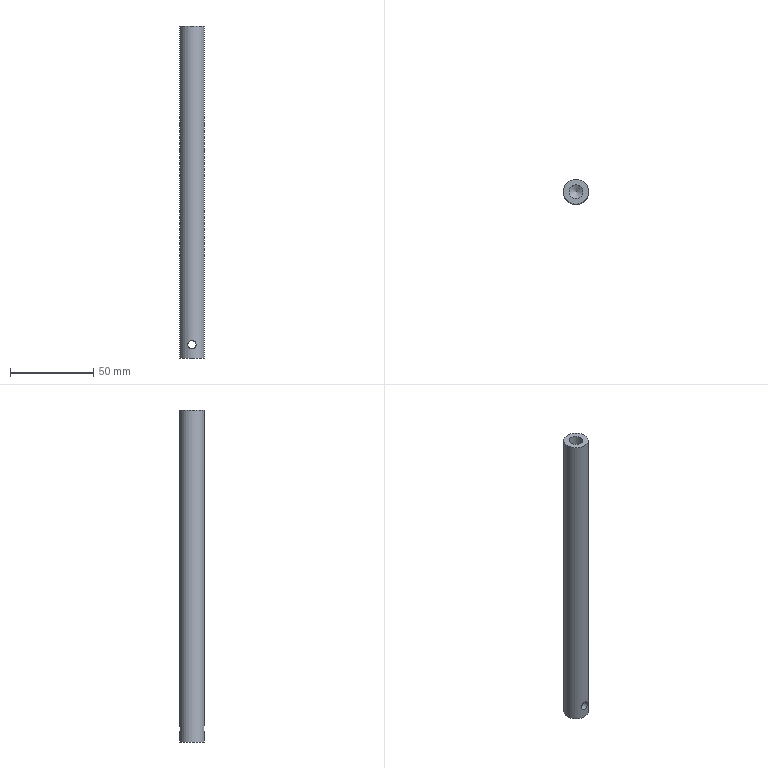Part | STEP file | axe for guide1-02 | 1 solid | 6 faces | box 15 x 15 x 200 mm | volume 33907 mm3 | spline 3 | plane 2 | cylinder 1 | commonest cylinder face diameters 15 x1
STEP:
#1=CARTESIAN_POINT('',(0.,0.,0.));
#2=DIRECTION('',(0.,0.,1.));
#3=DIRECTION('',(1.,0.,0.));
#4=AXIS2_PLACEMENT_3D('',#1,#2,#3);
#5=CARTESIAN_POINT('',(0.,7.5,10.5));
#6=VERTEX_POINT('',#5);
#7=CARTESIAN_POINT('',(0.,7.5,5.5));
#8=VERTEX_POINT('',#7);
#9=CARTESIAN_POINT('',(0.,7.5,10.5));
#10=CARTESIAN_POINT('',(-0.3165,7.5,10.5));
#11=CARTESIAN_POINT('',(-0.6524,7.478,10.436));
#12=CARTESIAN_POINT('',(-1.268,7.399,10.18));
#13=CARTESIAN_POINT('',(-1.547,7.342,9.988));
#14=CARTESIAN_POINT('',(-1.988,7.235,9.547));
#15=CARTESIAN_POINT('',(-2.18,7.177,9.268));
#16=CARTESIAN_POINT('',(-2.436,7.095,8.653));
#17=CARTESIAN_POINT('',(-2.5,7.071,8.317));
#18=CARTESIAN_POINT('',(-2.5,7.071,8.));
#19=CARTESIAN_POINT('',(-2.5,7.071,7.683));
#20=CARTESIAN_POINT('',(-2.436,7.095,7.347));
#21=CARTESIAN_POINT('',(-2.18,7.177,6.732));
#22=CARTESIAN_POINT('',(-1.988,7.235,6.453));
#23=CARTESIAN_POINT('',(-1.547,7.342,6.012));
#24=CARTESIAN_POINT('',(-1.268,7.399,5.82));
#25=CARTESIAN_POINT('',(-0.6524,7.478,5.564));
#26=CARTESIAN_POINT('',(-0.3165,7.5,5.5));
#27=CARTESIAN_POINT('',(0.,7.5,5.5));
#28=B_SPLINE_CURVE_WITH_KNOTS('',3,(#9,#10,#11,#12,#13,#14,#15,#16,#17,#18,#19,#20,#21,#22,#23,#24,#25,#26,#27),.UNSPECIFIED.,.F.,.F.,(4,2,2,2,3,2,2,2,4),(1.14,1.234,1.329,1.424,1.519,1.614,1.709,1.804,1.899),.UNSPECIFIED.);
#29=CARTESIAN_POINT('',(2.5,7.502,8.));
#30=CARTESIAN_POINT('',(2.5,7.502,5.5));
#31=CARTESIAN_POINT('',(0.,7.502,5.5));
#32=CARTESIAN_POINT('',(-2.5,7.502,5.5));
#33=CARTESIAN_POINT('',(-2.5,7.502,8.));
#34=CARTESIAN_POINT('',(-2.5,7.502,10.5));
#35=CARTESIAN_POINT('',(0.,7.502,10.5));
#36=CARTESIAN_POINT('',(2.5,7.502,10.5));
#37=CARTESIAN_POINT('',(2.5,7.502,8.));
#38=CARTESIAN_POINT('',(2.5,-7.502,8.));
#39=CARTESIAN_POINT('',(2.5,-7.502,5.5));
#40=CARTESIAN_POINT('',(0.,-7.502,5.5));
#41=CARTESIAN_POINT('',(-2.5,-7.502,5.5));
#42=CARTESIAN_POINT('',(-2.5,-7.502,8.));
#43=CARTESIAN_POINT('',(-2.5,-7.502,10.5));
#44=CARTESIAN_POINT('',(0.,-7.502,10.5));
#45=CARTESIAN_POINT('',(2.5,-7.502,10.5));
#46=CARTESIAN_POINT('',(2.5,-7.502,8.));
#47=(BOUNDED_SURFACE()B_SPLINE_SURFACE(1,2,((#29,#30,#31,#32,#33,#34,#35,#36,#37),(#38,#39,#40,#41,#42,#43,#44,#45,#46)),.UNSPECIFIED.,.F.,.T.,.F.)B_SPLINE_SURFACE_WITH_KNOTS((2,2),(1,2,2,2,2,2,1),(-80.449,-74.448),(-3.927,0.,3.927,7.854,11.781,15.708,19.635),.UNSPECIFIED.)GEOMETRIC_REPRESENTATION_ITEM()RATIONAL_B_SPLINE_SURFACE(((1.,0.7071,1.,0.7071,1.,0.7071,1.,0.7071,1.),(1.,0.7071,1.,0.7071,1.,0.7071,1.,0.7071,1.)))REPRESENTATION_ITEM('')SURFACE());
#48=CARTESIAN_POINT('',(-80.449,11.781));
#49=CARTESIAN_POINT('',(-80.449,11.717));
#50=CARTESIAN_POINT('',(-80.448,11.59));
#51=CARTESIAN_POINT('',(-80.446,11.4));
#52=CARTESIAN_POINT('',(-80.441,11.213));
#53=CARTESIAN_POINT('',(-80.436,11.028));
#54=CARTESIAN_POINT('',(-80.428,10.846));
#55=CARTESIAN_POINT('',(-80.42,10.667));
#56=CARTESIAN_POINT('',(-80.41,10.491));
#57=CARTESIAN_POINT('',(-80.399,10.317));
#58=CARTESIAN_POINT('',(-80.388,10.147));
#59=CARTESIAN_POINT('',(-80.376,9.98));
#60=CARTESIAN_POINT('',(-80.364,9.817));
#61=CARTESIAN_POINT('',(-80.352,9.655));
#62=CARTESIAN_POINT('',(-80.341,9.487));
#63=CARTESIAN_POINT('',(-80.329,9.317));
#64=CARTESIAN_POINT('',(-80.318,9.144));
#65=CARTESIAN_POINT('',(-80.308,8.968));
#66=CARTESIAN_POINT('',(-80.299,8.789));
#67=CARTESIAN_POINT('',(-80.291,8.607));
#68=CARTESIAN_POINT('',(-80.285,8.422));
#69=CARTESIAN_POINT('',(-80.281,8.235));
#70=CARTESIAN_POINT('',(-80.278,8.045));
#71=CARTESIAN_POINT('',(-80.277,7.854));
#72=CARTESIAN_POINT('',(-80.278,7.663));
#73=CARTESIAN_POINT('',(-80.281,7.473));
#74=CARTESIAN_POINT('',(-80.285,7.286));
#75=CARTESIAN_POINT('',(-80.291,7.101));
#76=CARTESIAN_POINT('',(-80.299,6.919));
#77=CARTESIAN_POINT('',(-80.308,6.74));
#78=CARTESIAN_POINT('',(-80.318,6.564));
#79=CARTESIAN_POINT('',(-80.329,6.391));
#80=CARTESIAN_POINT('',(-80.341,6.221));
#81=CARTESIAN_POINT('',(-80.352,6.053));
#82=CARTESIAN_POINT('',(-80.364,5.891));
#83=CARTESIAN_POINT('',(-80.376,5.728));
#84=CARTESIAN_POINT('',(-80.388,5.561));
#85=CARTESIAN_POINT('',(-80.399,5.391));
#86=CARTESIAN_POINT('',(-80.41,5.217));
#87=CARTESIAN_POINT('',(-80.42,5.041));
#88=CARTESIAN_POINT('',(-80.428,4.862));
#89=CARTESIAN_POINT('',(-80.436,4.68));
#90=CARTESIAN_POINT('',(-80.441,4.495));
#91=CARTESIAN_POINT('',(-80.446,4.308));
#92=CARTESIAN_POINT('',(-80.448,4.118));
#93=CARTESIAN_POINT('',(-80.449,3.991));
#94=CARTESIAN_POINT('',(-80.449,3.927));
#95=B_SPLINE_CURVE_WITH_KNOTS('',3,(#48,#49,#50,#51,#52,#53,#54,#55,#56,#57,#58,#59,#60,#61,#62,#63,#64,#65,#66,#67,#68,#69,#70,#71,#72,#73,#74,#75,#76,#77,#78,#79,#80,#81,#82,#83,#84,#85,#86,#87,#88,#89,#90,#91,#92,#93,#94),.UNSPECIFIED.,.F.,.F.,(4,1,1,1,1,1,1,1,1,1,1,1,1,1,1,1,1,1,1,1,1,1,1,1,1,1,1,1,1,1,1,1,1,1,1,1,1,1,1,1,1,1,1,1,4),(1.14,1.157,1.174,1.191,1.209,1.226,1.243,1.26,1.278,1.295,1.312,1.329,1.347,1.364,1.381,1.399,1.416,1.433,1.45,1.468,1.485,1.502,1.519,1.537,1.554,1.571,1.588,1.606,1.623,1.64,1.658,1.675,1.692,1.709,1.727,1.744,1.761,1.778,1.796,1.813,1.83,1.847,1.865,1.882,1.899),.QUASI_UNIFORM_KNOTS.);
#96=(GEOMETRIC_REPRESENTATION_CONTEXT(2)PARAMETRIC_REPRESENTATION_CONTEXT()REPRESENTATION_CONTEXT('',''));
#97=DEFINITIONAL_REPRESENTATION('',(#95),#96);
#98=PCURVE('',#47,#97);
#99=CARTESIAN_POINT('',(0.,0.,0.));
#100=DIRECTION('',(0.,0.,1.));
#101=DIRECTION('',(-1.,0.,0.));
#102=AXIS2_PLACEMENT_3D('',#99,#100,#101);
#103=CYLINDRICAL_SURFACE('',#102,7.5);
#104=CARTESIAN_POINT('',(4.712,10.5));
#105=CARTESIAN_POINT('',(4.72,10.5));
#106=CARTESIAN_POINT('',(4.736,10.496));
#107=CARTESIAN_POINT('',(4.759,10.477));
#108=CARTESIAN_POINT('',(4.783,10.445));
#109=CARTESIAN_POINT('',(4.806,10.401));
#110=CARTESIAN_POINT('',(4.83,10.344));
#111=CARTESIAN_POINT('',(4.852,10.274));
#112=CARTESIAN_POINT('',(4.874,10.192));
#113=CARTESIAN_POINT('',(4.895,10.099));
#114=CARTESIAN_POINT('',(4.915,9.997));
#115=CARTESIAN_POINT('',(4.933,9.886));
#116=CARTESIAN_POINT('',(4.951,9.769));
#117=CARTESIAN_POINT('',(4.967,9.643));
#118=CARTESIAN_POINT('',(4.982,9.506));
#119=CARTESIAN_POINT('',(4.996,9.36));
#120=CARTESIAN_POINT('',(5.009,9.206));
#121=CARTESIAN_POINT('',(5.02,9.044));
#122=CARTESIAN_POINT('',(5.03,8.876));
#123=CARTESIAN_POINT('',(5.038,8.703));
#124=CARTESIAN_POINT('',(5.044,8.528));
#125=CARTESIAN_POINT('',(5.049,8.351));
#126=CARTESIAN_POINT('',(5.052,8.174));
#127=CARTESIAN_POINT('',(5.053,8.));
#128=CARTESIAN_POINT('',(5.052,7.826));
#129=CARTESIAN_POINT('',(5.049,7.649));
#130=CARTESIAN_POINT('',(5.044,7.472));
#131=CARTESIAN_POINT('',(5.038,7.297));
#132=CARTESIAN_POINT('',(5.03,7.124));
#133=CARTESIAN_POINT('',(5.02,6.956));
#134=CARTESIAN_POINT('',(5.009,6.794));
#135=CARTESIAN_POINT('',(4.996,6.64));
#136=CARTESIAN_POINT('',(4.982,6.494));
#137=CARTESIAN_POINT('',(4.967,6.357));
#138=CARTESIAN_POINT('',(4.951,6.231));
#139=CARTESIAN_POINT('',(4.933,6.114));
#140=CARTESIAN_POINT('',(4.915,6.003));
#141=CARTESIAN_POINT('',(4.895,5.901));
#142=CARTESIAN_POINT('',(4.874,5.808));
#143=CARTESIAN_POINT('',(4.852,5.726));
#144=CARTESIAN_POINT('',(4.83,5.656));
#145=CARTESIAN_POINT('',(4.806,5.599));
#146=CARTESIAN_POINT('',(4.783,5.555));
#147=CARTESIAN_POINT('',(4.759,5.523));
#148=CARTESIAN_POINT('',(4.736,5.504));
#149=CARTESIAN_POINT('',(4.72,5.5));
#150=CARTESIAN_POINT('',(4.712,5.5));
#151=B_SPLINE_CURVE_WITH_KNOTS('',3,(#104,#105,#106,#107,#108,#109,#110,#111,#112,#113,#114,#115,#116,#117,#118,#119,#120,#121,#122,#123,#124,#125,#126,#127,#128,#129,#130,#131,#132,#133,#134,#135,#136,#137,#138,#139,#140,#141,#142,#143,#144,#145,#146,#147,#148,#149,#150),.UNSPECIFIED.,.F.,.F.,(4,1,1,1,1,1,1,1,1,1,1,1,1,1,1,1,1,1,1,1,1,1,1,1,1,1,1,1,1,1,1,1,1,1,1,1,1,1,1,1,1,1,1,1,4),(1.14,1.157,1.174,1.191,1.209,1.226,1.243,1.26,1.278,1.295,1.312,1.329,1.347,1.364,1.381,1.399,1.416,1.433,1.45,1.468,1.485,1.502,1.519,1.537,1.554,1.571,1.588,1.606,1.623,1.64,1.658,1.675,1.692,1.709,1.727,1.744,1.761,1.778,1.796,1.813,1.83,1.847,1.865,1.882,1.899),.QUASI_UNIFORM_KNOTS.);
#152=(GEOMETRIC_REPRESENTATION_CONTEXT(2)PARAMETRIC_REPRESENTATION_CONTEXT()REPRESENTATION_CONTEXT('',''));
#153=DEFINITIONAL_REPRESENTATION('',(#151),#152);
#154=PCURVE('',#103,#153);
#155=SURFACE_CURVE('',#28,(#98,#154),.PCURVE_S1.);
#156=EDGE_CURVE('',#6,#8,#155,.T.);
#157=ORIENTED_EDGE('',*,*,#156,.T.);
#158=CARTESIAN_POINT('',(0.,-7.5,5.5));
#159=VERTEX_POINT('',#158);
#160=CARTESIAN_POINT('',(0.,7.5,5.5));
#161=CARTESIAN_POINT('',(0.,-7.5,5.5));
#162=B_SPLINE_CURVE_WITH_KNOTS('',1,(#160,#161),.UNSPECIFIED.,.F.,.F.,(2,2),(-80.449,-74.449),.PIECEWISE_BEZIER_KNOTS.);
#163=CARTESIAN_POINT('',(0.,3.927));
#164=DIRECTION('',(1.,0.));
#165=VECTOR('',#164,1.);
#166=LINE('',#163,#165);
#167=(GEOMETRIC_REPRESENTATION_CONTEXT(2)PARAMETRIC_REPRESENTATION_CONTEXT()REPRESENTATION_CONTEXT('',''));
#168=DEFINITIONAL_REPRESENTATION('',(#166),#167);
#169=PCURVE('',#47,#168);
#170=CARTESIAN_POINT('',(0.,19.635));
#171=DIRECTION('',(1.,0.));
#172=VECTOR('',#171,1.);
#173=LINE('',#170,#172);
#174=(GEOMETRIC_REPRESENTATION_CONTEXT(2)PARAMETRIC_REPRESENTATION_CONTEXT()REPRESENTATION_CONTEXT('',''));
#175=DEFINITIONAL_REPRESENTATION('',(#173),#174);
#176=PCURVE('',#47,#175);
#177=SEAM_CURVE('',#162,(#169,#176),.PCURVE_S1.);
#178=EDGE_CURVE('',#8,#159,#177,.T.);
#179=ORIENTED_EDGE('',*,*,#178,.T.);
#180=CARTESIAN_POINT('',(-2.5,-7.071,8.));
#181=VERTEX_POINT('',#180);
#182=CARTESIAN_POINT('',(-2.5,-7.071,8.));
#183=CARTESIAN_POINT('',(-2.5,-7.071,8.317));
#184=CARTESIAN_POINT('',(-2.436,-7.095,8.653));
#185=CARTESIAN_POINT('',(-2.18,-7.177,9.268));
#186=CARTESIAN_POINT('',(-1.988,-7.235,9.547));
#187=CARTESIAN_POINT('',(-1.547,-7.342,9.988));
#188=CARTESIAN_POINT('',(-1.268,-7.399,10.18));
#189=CARTESIAN_POINT('',(-0.6524,-7.478,10.436));
#190=CARTESIAN_POINT('',(-0.3165,-7.5,10.5));
#191=CARTESIAN_POINT('',(0.3165,-7.5,10.5));
#192=CARTESIAN_POINT('',(0.6524,-7.478,10.436));
#193=CARTESIAN_POINT('',(1.268,-7.399,10.18));
#194=CARTESIAN_POINT('',(1.547,-7.342,9.988));
#195=CARTESIAN_POINT('',(1.988,-7.235,9.547));
#196=CARTESIAN_POINT('',(2.18,-7.177,9.268));
#197=CARTESIAN_POINT('',(2.436,-7.095,8.653));
#198=CARTESIAN_POINT('',(2.5,-7.071,8.317));
#199=CARTESIAN_POINT('',(2.5,-7.071,7.683));
#200=CARTESIAN_POINT('',(2.436,-7.095,7.347));
#201=CARTESIAN_POINT('',(2.18,-7.177,6.732));
#202=CARTESIAN_POINT('',(1.988,-7.235,6.453));
#203=CARTESIAN_POINT('',(1.547,-7.342,6.012));
#204=CARTESIAN_POINT('',(1.268,-7.399,5.82));
#205=CARTESIAN_POINT('',(0.6524,-7.478,5.564));
#206=CARTESIAN_POINT('',(0.3165,-7.5,5.5));
#207=CARTESIAN_POINT('',(-0.3165,-7.5,5.5));
#208=CARTESIAN_POINT('',(-0.6524,-7.478,5.564));
#209=CARTESIAN_POINT('',(-1.268,-7.399,5.82));
#210=CARTESIAN_POINT('',(-1.547,-7.342,6.012));
#211=CARTESIAN_POINT('',(-1.988,-7.235,6.453));
#212=CARTESIAN_POINT('',(-2.18,-7.177,6.732));
#213=CARTESIAN_POINT('',(-2.436,-7.095,7.347));
#214=CARTESIAN_POINT('',(-2.5,-7.071,7.683));
#215=CARTESIAN_POINT('',(-2.5,-7.071,8.));
#216=B_SPLINE_CURVE_WITH_KNOTS('',3,(#182,#183,#184,#185,#186,#187,#188,#189,#190,#191,#192,#193,#194,#195,#196,#197,#198,#199,#200,#201,#202,#203,#204,#205,#206,#207,#208,#209,#210,#211,#212,#213,#214,#215),.UNSPECIFIED.,.T.,.F.,(1,3,2,2,2,2,2,2,2,2,2,2,2,2,2,2,2,3,1),(-0.09498,0.,0.09498,0.19,0.2849,0.3799,0.4748,0.5697,0.6647,0.7597,0.8547,0.9497,1.045,1.14,1.234,1.329,1.424,1.519,1.614),.UNSPECIFIED.);
#217=CARTESIAN_POINT('',(-74.62,-7.854));
#218=CARTESIAN_POINT('',(-74.62,-7.769));
#219=CARTESIAN_POINT('',(-74.619,-7.599));
#220=CARTESIAN_POINT('',(-74.614,-7.348));
#221=CARTESIAN_POINT('',(-74.607,-7.101));
#222=CARTESIAN_POINT('',(-74.596,-6.859));
#223=CARTESIAN_POINT('',(-74.583,-6.622));
#224=CARTESIAN_POINT('',(-74.569,-6.391));
#225=CARTESIAN_POINT('',(-74.553,-6.164));
#226=CARTESIAN_POINT('',(-74.537,-5.944));
#227=CARTESIAN_POINT('',(-74.522,-5.729));
#228=CARTESIAN_POINT('',(-74.506,-5.505));
#229=CARTESIAN_POINT('',(-74.491,-5.276));
#230=CARTESIAN_POINT('',(-74.478,-5.041));
#231=CARTESIAN_POINT('',(-74.466,-4.802));
#232=CARTESIAN_POINT('',(-74.458,-4.557));
#233=CARTESIAN_POINT('',(-74.452,-4.308));
#234=CARTESIAN_POINT('',(-74.449,-4.055));
#235=CARTESIAN_POINT('',(-74.449,-3.799));
#236=CARTESIAN_POINT('',(-74.452,-3.546));
#237=CARTESIAN_POINT('',(-74.458,-3.297));
#238=CARTESIAN_POINT('',(-74.466,-3.052));
#239=CARTESIAN_POINT('',(-74.478,-2.813));
#240=CARTESIAN_POINT('',(-74.491,-2.578));
#241=CARTESIAN_POINT('',(-74.506,-2.349));
#242=CARTESIAN_POINT('',(-74.522,-2.125));
#243=CARTESIAN_POINT('',(-74.537,-1.91));
#244=CARTESIAN_POINT('',(-74.553,-1.69));
#245=CARTESIAN_POINT('',(-74.569,-1.463));
#246=CARTESIAN_POINT('',(-74.583,-1.232));
#247=CARTESIAN_POINT('',(-74.596,-0.9949));
#248=CARTESIAN_POINT('',(-74.607,-0.7531));
#249=CARTESIAN_POINT('',(-74.614,-0.5062));
#250=CARTESIAN_POINT('',(-74.619,-0.2551));
#251=CARTESIAN_POINT('',(-74.621,0.));
#252=CARTESIAN_POINT('',(-74.619,0.2551));
#253=CARTESIAN_POINT('',(-74.614,0.5062));
#254=CARTESIAN_POINT('',(-74.607,0.7531));
#255=CARTESIAN_POINT('',(-74.596,0.9949));
#256=CARTESIAN_POINT('',(-74.583,1.232));
#257=CARTESIAN_POINT('',(-74.569,1.463));
#258=CARTESIAN_POINT('',(-74.553,1.69));
#259=CARTESIAN_POINT('',(-74.537,1.91));
#260=CARTESIAN_POINT('',(-74.522,2.125));
#261=CARTESIAN_POINT('',(-74.506,2.349));
#262=CARTESIAN_POINT('',(-74.491,2.578));
#263=CARTESIAN_POINT('',(-74.478,2.813));
#264=CARTESIAN_POINT('',(-74.466,3.052));
#265=CARTESIAN_POINT('',(-74.458,3.297));
#266=CARTESIAN_POINT('',(-74.452,3.546));
#267=CARTESIAN_POINT('',(-74.449,3.799));
#268=CARTESIAN_POINT('',(-74.449,4.055));
#269=CARTESIAN_POINT('',(-74.452,4.308));
#270=CARTESIAN_POINT('',(-74.458,4.557));
#271=CARTESIAN_POINT('',(-74.466,4.802));
#272=CARTESIAN_POINT('',(-74.478,5.041));
#273=CARTESIAN_POINT('',(-74.491,5.276));
#274=CARTESIAN_POINT('',(-74.506,5.505));
#275=CARTESIAN_POINT('',(-74.522,5.729));
#276=CARTESIAN_POINT('',(-74.537,5.944));
#277=CARTESIAN_POINT('',(-74.553,6.164));
#278=CARTESIAN_POINT('',(-74.569,6.391));
#279=CARTESIAN_POINT('',(-74.583,6.622));
#280=CARTESIAN_POINT('',(-74.596,6.859));
#281=CARTESIAN_POINT('',(-74.607,7.101));
#282=CARTESIAN_POINT('',(-74.614,7.348));
#283=CARTESIAN_POINT('',(-74.619,7.599));
#284=CARTESIAN_POINT('',(-74.62,7.769));
#285=CARTESIAN_POINT('',(-74.62,7.854));
#286=B_SPLINE_CURVE_WITH_KNOTS('',3,(#217,#218,#219,#220,#221,#222,#223,#224,#225,#226,#227,#228,#229,#230,#231,#232,#233,#234,#235,#236,#237,#238,#239,#240,#241,#242,#243,#244,#245,#246,#247,#248,#249,#250,#251,#252,#253,#254,#255,#256,#257,#258,#259,#260,#261,#262,#263,#264,#265,#266,#267,#268,#269,#270,#271,#272,#273,#274,#275,#276,#277,#278,#279,#280,#281,#282,#283,#284,#285),.UNSPECIFIED.,.F.,.F.,(4,1,1,1,1,1,1,1,1,1,1,1,1,1,1,1,1,1,1,1,1,1,1,1,1,1,1,1,1,1,1,1,1,1,1,1,1,1,1,1,1,1,1,1,1,1,1,1,1,1,1,1,1,1,1,1,1,1,1,1,1,1,1,1,1,1,4),(0.,0.02302,0.04604,0.06906,0.09208,0.1151,0.1381,0.1611,0.1842,0.2072,0.2302,0.2532,0.2763,0.2993,0.3223,0.3453,0.3683,0.3914,0.4144,0.4374,0.4604,0.4834,0.5065,0.5295,0.5525,0.5755,0.5986,0.6216,0.6446,0.6676,0.6906,0.7137,0.7367,0.7597,0.7827,0.8057,0.8288,0.8518,0.8748,0.8978,0.9208,0.9439,0.9669,0.9899,1.013,1.036,1.059,1.082,1.105,1.128,1.151,1.174,1.197,1.22,1.243,1.266,1.289,1.312,1.335,1.358,1.381,1.404,1.427,1.45,1.473,1.496,1.519),.QUASI_UNIFORM_KNOTS.);
#287=(GEOMETRIC_REPRESENTATION_CONTEXT(2)PARAMETRIC_REPRESENTATION_CONTEXT()REPRESENTATION_CONTEXT('',''));
#288=DEFINITIONAL_REPRESENTATION('',(#286),#287);
#289=PCURVE('',#47,#288);
#290=CARTESIAN_POINT('',(7.854,5.5));
#291=CARTESIAN_POINT('',(7.846,5.5));
#292=CARTESIAN_POINT('',(7.831,5.504));
#293=CARTESIAN_POINT('',(7.807,5.523));
#294=CARTESIAN_POINT('',(7.784,5.555));
#295=CARTESIAN_POINT('',(7.76,5.599));
#296=CARTESIAN_POINT('',(7.737,5.656));
#297=CARTESIAN_POINT('',(7.714,5.726));
#298=CARTESIAN_POINT('',(7.692,5.808));
#299=CARTESIAN_POINT('',(7.672,5.901));
#300=CARTESIAN_POINT('',(7.652,6.003));
#301=CARTESIAN_POINT('',(7.633,6.114));
#302=CARTESIAN_POINT('',(7.616,6.231));
#303=CARTESIAN_POINT('',(7.6,6.357));
#304=CARTESIAN_POINT('',(7.584,6.494));
#305=CARTESIAN_POINT('',(7.57,6.64));
#306=CARTESIAN_POINT('',(7.557,6.794));
#307=CARTESIAN_POINT('',(7.546,6.956));
#308=CARTESIAN_POINT('',(7.536,7.124));
#309=CARTESIAN_POINT('',(7.528,7.297));
#310=CARTESIAN_POINT('',(7.522,7.472));
#311=CARTESIAN_POINT('',(7.517,7.649));
#312=CARTESIAN_POINT('',(7.515,7.826));
#313=CARTESIAN_POINT('',(7.514,7.942));
#314=CARTESIAN_POINT('',(7.514,8.));
#315=B_SPLINE_CURVE_WITH_KNOTS('',3,(#290,#291,#292,#293,#294,#295,#296,#297,#298,#299,#300,#301,#302,#303,#304,#305,#306,#307,#308,#309,#310,#311,#312,#313,#314),.UNSPECIFIED.,.F.,.F.,(4,1,1,1,1,1,1,1,1,1,1,1,1,1,1,1,1,1,1,1,1,1,4),(1.14,1.157,1.174,1.191,1.209,1.226,1.243,1.26,1.278,1.295,1.312,1.329,1.347,1.364,1.381,1.399,1.416,1.433,1.45,1.468,1.485,1.502,1.519),.QUASI_UNIFORM_KNOTS.);
#316=(GEOMETRIC_REPRESENTATION_CONTEXT(2)PARAMETRIC_REPRESENTATION_CONTEXT()REPRESENTATION_CONTEXT('',''));
#317=DEFINITIONAL_REPRESENTATION('',(#315),#316);
#318=PCURVE('',#103,#317);
#319=SURFACE_CURVE('',#216,(#289,#318),.PCURVE_S1.);
#320=EDGE_CURVE('',#159,#181,#319,.T.);
#321=ORIENTED_EDGE('',*,*,#320,.T.);
#322=CARTESIAN_POINT('',(-2.5,-7.071,8.));
#323=CARTESIAN_POINT('',(-2.5,-7.071,8.317));
#324=CARTESIAN_POINT('',(-2.436,-7.095,8.653));
#325=CARTESIAN_POINT('',(-2.18,-7.177,9.268));
#326=CARTESIAN_POINT('',(-1.988,-7.235,9.547));
#327=CARTESIAN_POINT('',(-1.547,-7.342,9.988));
#328=CARTESIAN_POINT('',(-1.268,-7.399,10.18));
#329=CARTESIAN_POINT('',(-0.6524,-7.478,10.436));
#330=CARTESIAN_POINT('',(-0.3165,-7.5,10.5));
#331=CARTESIAN_POINT('',(0.3165,-7.5,10.5));
#332=CARTESIAN_POINT('',(0.6524,-7.478,10.436));
#333=CARTESIAN_POINT('',(1.268,-7.399,10.18));
#334=CARTESIAN_POINT('',(1.547,-7.342,9.988));
#335=CARTESIAN_POINT('',(1.988,-7.235,9.547));
#336=CARTESIAN_POINT('',(2.18,-7.177,9.268));
#337=CARTESIAN_POINT('',(2.436,-7.095,8.653));
#338=CARTESIAN_POINT('',(2.5,-7.071,8.317));
#339=CARTESIAN_POINT('',(2.5,-7.071,7.683));
#340=CARTESIAN_POINT('',(2.436,-7.095,7.347));
#341=CARTESIAN_POINT('',(2.18,-7.177,6.732));
#342=CARTESIAN_POINT('',(1.988,-7.235,6.453));
#343=CARTESIAN_POINT('',(1.547,-7.342,6.012));
#344=CARTESIAN_POINT('',(1.268,-7.399,5.82));
#345=CARTESIAN_POINT('',(0.6524,-7.478,5.564));
#346=CARTESIAN_POINT('',(0.3165,-7.5,5.5));
#347=CARTESIAN_POINT('',(-0.3165,-7.5,5.5));
#348=CARTESIAN_POINT('',(-0.6524,-7.478,5.564));
#349=CARTESIAN_POINT('',(-1.268,-7.399,5.82));
#350=CARTESIAN_POINT('',(-1.547,-7.342,6.012));
#351=CARTESIAN_POINT('',(-1.988,-7.235,6.453));
#352=CARTESIAN_POINT('',(-2.18,-7.177,6.732));
#353=CARTESIAN_POINT('',(-2.436,-7.095,7.347));
#354=CARTESIAN_POINT('',(-2.5,-7.071,7.683));
#355=CARTESIAN_POINT('',(-2.5,-7.071,8.));
#356=B_SPLINE_CURVE_WITH_KNOTS('',3,(#322,#323,#324,#325,#326,#327,#328,#329,#330,#331,#332,#333,#334,#335,#336,#337,#338,#339,#340,#341,#342,#343,#344,#345,#346,#347,#348,#349,#350,#351,#352,#353,#354,#355),.UNSPECIFIED.,.T.,.F.,(1,3,2,2,2,2,2,2,2,2,2,2,2,2,2,2,2,3,1),(-0.09498,0.,0.09498,0.19,0.2849,0.3799,0.4748,0.5697,0.6647,0.7597,0.8547,0.9497,1.045,1.14,1.234,1.329,1.424,1.519,1.614),.UNSPECIFIED.);
#357=CARTESIAN_POINT('',(-74.62,7.854));
#358=CARTESIAN_POINT('',(-74.62,7.939));
#359=CARTESIAN_POINT('',(-74.619,8.109));
#360=CARTESIAN_POINT('',(-74.614,8.36));
#361=CARTESIAN_POINT('',(-74.607,8.607));
#362=CARTESIAN_POINT('',(-74.596,8.849));
#363=CARTESIAN_POINT('',(-74.583,9.086));
#364=CARTESIAN_POINT('',(-74.569,9.317));
#365=CARTESIAN_POINT('',(-74.553,9.544));
#366=CARTESIAN_POINT('',(-74.537,9.764));
#367=CARTESIAN_POINT('',(-74.522,9.979));
#368=CARTESIAN_POINT('',(-74.506,10.203));
#369=CARTESIAN_POINT('',(-74.491,10.432));
#370=CARTESIAN_POINT('',(-74.478,10.667));
#371=CARTESIAN_POINT('',(-74.466,10.906));
#372=CARTESIAN_POINT('',(-74.458,11.151));
#373=CARTESIAN_POINT('',(-74.452,11.4));
#374=CARTESIAN_POINT('',(-74.449,11.653));
#375=CARTESIAN_POINT('',(-74.449,11.909));
#376=CARTESIAN_POINT('',(-74.452,12.162));
#377=CARTESIAN_POINT('',(-74.458,12.411));
#378=CARTESIAN_POINT('',(-74.466,12.656));
#379=CARTESIAN_POINT('',(-74.478,12.895));
#380=CARTESIAN_POINT('',(-74.491,13.13));
#381=CARTESIAN_POINT('',(-74.506,13.359));
#382=CARTESIAN_POINT('',(-74.522,13.583));
#383=CARTESIAN_POINT('',(-74.537,13.798));
#384=CARTESIAN_POINT('',(-74.553,14.018));
#385=CARTESIAN_POINT('',(-74.569,14.245));
#386=CARTESIAN_POINT('',(-74.583,14.476));
#387=CARTESIAN_POINT('',(-74.596,14.713));
#388=CARTESIAN_POINT('',(-74.607,14.955));
#389=CARTESIAN_POINT('',(-74.614,15.202));
#390=CARTESIAN_POINT('',(-74.619,15.453));
#391=CARTESIAN_POINT('',(-74.621,15.708));
#392=CARTESIAN_POINT('',(-74.619,15.963));
#393=CARTESIAN_POINT('',(-74.614,16.214));
#394=CARTESIAN_POINT('',(-74.607,16.461));
#395=CARTESIAN_POINT('',(-74.596,16.703));
#396=CARTESIAN_POINT('',(-74.583,16.94));
#397=CARTESIAN_POINT('',(-74.569,17.171));
#398=CARTESIAN_POINT('',(-74.553,17.398));
#399=CARTESIAN_POINT('',(-74.537,17.618));
#400=CARTESIAN_POINT('',(-74.522,17.833));
#401=CARTESIAN_POINT('',(-74.506,18.057));
#402=CARTESIAN_POINT('',(-74.491,18.286));
#403=CARTESIAN_POINT('',(-74.478,18.521));
#404=CARTESIAN_POINT('',(-74.466,18.76));
#405=CARTESIAN_POINT('',(-74.458,19.005));
#406=CARTESIAN_POINT('',(-74.452,19.254));
#407=CARTESIAN_POINT('',(-74.449,19.507));
#408=CARTESIAN_POINT('',(-74.449,19.763));
#409=CARTESIAN_POINT('',(-74.452,20.016));
#410=CARTESIAN_POINT('',(-74.458,20.265));
#411=CARTESIAN_POINT('',(-74.466,20.51));
#412=CARTESIAN_POINT('',(-74.478,20.749));
#413=CARTESIAN_POINT('',(-74.491,20.984));
#414=CARTESIAN_POINT('',(-74.506,21.213));
#415=CARTESIAN_POINT('',(-74.522,21.437));
#416=CARTESIAN_POINT('',(-74.537,21.652));
#417=CARTESIAN_POINT('',(-74.553,21.872));
#418=CARTESIAN_POINT('',(-74.569,22.098));
#419=CARTESIAN_POINT('',(-74.583,22.33));
#420=CARTESIAN_POINT('',(-74.596,22.567));
#421=CARTESIAN_POINT('',(-74.607,22.809));
#422=CARTESIAN_POINT('',(-74.614,23.056));
#423=CARTESIAN_POINT('',(-74.619,23.307));
#424=CARTESIAN_POINT('',(-74.62,23.477));
#425=CARTESIAN_POINT('',(-74.62,23.562));
#426=B_SPLINE_CURVE_WITH_KNOTS('',3,(#357,#358,#359,#360,#361,#362,#363,#364,#365,#366,#367,#368,#369,#370,#371,#372,#373,#374,#375,#376,#377,#378,#379,#380,#381,#382,#383,#384,#385,#386,#387,#388,#389,#390,#391,#392,#393,#394,#395,#396,#397,#398,#399,#400,#401,#402,#403,#404,#405,#406,#407,#408,#409,#410,#411,#412,#413,#414,#415,#416,#417,#418,#419,#420,#421,#422,#423,#424,#425),.UNSPECIFIED.,.F.,.F.,(4,1,1,1,1,1,1,1,1,1,1,1,1,1,1,1,1,1,1,1,1,1,1,1,1,1,1,1,1,1,1,1,1,1,1,1,1,1,1,1,1,1,1,1,1,1,1,1,1,1,1,1,1,1,1,1,1,1,1,1,1,1,1,1,1,1,4),(0.,0.02302,0.04604,0.06906,0.09208,0.1151,0.1381,0.1611,0.1842,0.2072,0.2302,0.2532,0.2763,0.2993,0.3223,0.3453,0.3683,0.3914,0.4144,0.4374,0.4604,0.4834,0.5065,0.5295,0.5525,0.5755,0.5986,0.6216,0.6446,0.6676,0.6906,0.7137,0.7367,0.7597,0.7827,0.8057,0.8288,0.8518,0.8748,0.8978,0.9208,0.9439,0.9669,0.9899,1.013,1.036,1.059,1.082,1.105,1.128,1.151,1.174,1.197,1.22,1.243,1.266,1.289,1.312,1.335,1.358,1.381,1.404,1.427,1.45,1.473,1.496,1.519),.QUASI_UNIFORM_KNOTS.);
#427=(GEOMETRIC_REPRESENTATION_CONTEXT(2)PARAMETRIC_REPRESENTATION_CONTEXT()REPRESENTATION_CONTEXT('',''));
#428=DEFINITIONAL_REPRESENTATION('',(#426),#427);
#429=PCURVE('',#47,#428);
#430=CARTESIAN_POINT('',(7.514,8.));
#431=CARTESIAN_POINT('',(7.514,8.058));
#432=CARTESIAN_POINT('',(7.515,8.174));
#433=CARTESIAN_POINT('',(7.517,8.351));
#434=CARTESIAN_POINT('',(7.522,8.528));
#435=CARTESIAN_POINT('',(7.528,8.703));
#436=CARTESIAN_POINT('',(7.536,8.876));
#437=CARTESIAN_POINT('',(7.546,9.044));
#438=CARTESIAN_POINT('',(7.557,9.206));
#439=CARTESIAN_POINT('',(7.57,9.36));
#440=CARTESIAN_POINT('',(7.584,9.506));
#441=CARTESIAN_POINT('',(7.6,9.643));
#442=CARTESIAN_POINT('',(7.616,9.769));
#443=CARTESIAN_POINT('',(7.633,9.886));
#444=CARTESIAN_POINT('',(7.652,9.997));
#445=CARTESIAN_POINT('',(7.672,10.099));
#446=CARTESIAN_POINT('',(7.692,10.192));
#447=CARTESIAN_POINT('',(7.714,10.274));
#448=CARTESIAN_POINT('',(7.737,10.344));
#449=CARTESIAN_POINT('',(7.76,10.401));
#450=CARTESIAN_POINT('',(7.784,10.445));
#451=CARTESIAN_POINT('',(7.807,10.477));
#452=CARTESIAN_POINT('',(7.831,10.496));
#453=CARTESIAN_POINT('',(7.854,10.502));
#454=CARTESIAN_POINT('',(7.877,10.496));
#455=CARTESIAN_POINT('',(7.901,10.477));
#456=CARTESIAN_POINT('',(7.924,10.445));
#457=CARTESIAN_POINT('',(7.948,10.401));
#458=CARTESIAN_POINT('',(7.971,10.344));
#459=CARTESIAN_POINT('',(7.994,10.274));
#460=CARTESIAN_POINT('',(8.016,10.192));
#461=CARTESIAN_POINT('',(8.036,10.099));
#462=CARTESIAN_POINT('',(8.056,9.997));
#463=CARTESIAN_POINT('',(8.075,9.886));
#464=CARTESIAN_POINT('',(8.092,9.769));
#465=CARTESIAN_POINT('',(8.108,9.643));
#466=CARTESIAN_POINT('',(8.123,9.506));
#467=CARTESIAN_POINT('',(8.138,9.36));
#468=CARTESIAN_POINT('',(8.151,9.206));
#469=CARTESIAN_POINT('',(8.162,9.044));
#470=CARTESIAN_POINT('',(8.172,8.876));
#471=CARTESIAN_POINT('',(8.18,8.703));
#472=CARTESIAN_POINT('',(8.186,8.528));
#473=CARTESIAN_POINT('',(8.191,8.351));
#474=CARTESIAN_POINT('',(8.193,8.174));
#475=CARTESIAN_POINT('',(8.194,8.));
#476=CARTESIAN_POINT('',(8.193,7.826));
#477=CARTESIAN_POINT('',(8.191,7.649));
#478=CARTESIAN_POINT('',(8.186,7.472));
#479=CARTESIAN_POINT('',(8.18,7.297));
#480=CARTESIAN_POINT('',(8.172,7.124));
#481=CARTESIAN_POINT('',(8.162,6.956));
#482=CARTESIAN_POINT('',(8.151,6.794));
#483=CARTESIAN_POINT('',(8.138,6.64));
#484=CARTESIAN_POINT('',(8.123,6.494));
#485=CARTESIAN_POINT('',(8.108,6.357));
#486=CARTESIAN_POINT('',(8.092,6.231));
#487=CARTESIAN_POINT('',(8.075,6.114));
#488=CARTESIAN_POINT('',(8.056,6.003));
#489=CARTESIAN_POINT('',(8.036,5.901));
#490=CARTESIAN_POINT('',(8.016,5.808));
#491=CARTESIAN_POINT('',(7.994,5.726));
#492=CARTESIAN_POINT('',(7.971,5.656));
#493=CARTESIAN_POINT('',(7.948,5.599));
#494=CARTESIAN_POINT('',(7.924,5.555));
#495=CARTESIAN_POINT('',(7.901,5.523));
#496=CARTESIAN_POINT('',(7.877,5.504));
#497=CARTESIAN_POINT('',(7.862,5.5));
#498=CARTESIAN_POINT('',(7.854,5.5));
#499=B_SPLINE_CURVE_WITH_KNOTS('',3,(#430,#431,#432,#433,#434,#435,#436,#437,#438,#439,#440,#441,#442,#443,#444,#445,#446,#447,#448,#449,#450,#451,#452,#453,#454,#455,#456,#457,#458,#459,#460,#461,#462,#463,#464,#465,#466,#467,#468,#469,#470,#471,#472,#473,#474,#475,#476,#477,#478,#479,#480,#481,#482,#483,#484,#485,#486,#487,#488,#489,#490,#491,#492,#493,#494,#495,#496,#497,#498),.UNSPECIFIED.,.F.,.F.,(4,1,1,1,1,1,1,1,1,1,1,1,1,1,1,1,1,1,1,1,1,1,1,1,1,1,1,1,1,1,1,1,1,1,1,1,1,1,1,1,1,1,1,1,1,1,1,1,1,1,1,1,1,1,1,1,1,1,1,1,1,1,1,1,1,1,4),(0.,0.01727,0.03453,0.0518,0.06906,0.08633,0.1036,0.1209,0.1381,0.1554,0.1727,0.1899,0.2072,0.2245,0.2417,0.259,0.2763,0.2935,0.3108,0.3281,0.3453,0.3626,0.3799,0.3971,0.4144,0.4316,0.4489,0.4662,0.4834,0.5007,0.518,0.5352,0.5525,0.5698,0.587,0.6043,0.6216,0.6388,0.6561,0.6734,0.6906,0.7079,0.7252,0.7424,0.7597,0.777,0.7942,0.8115,0.8288,0.846,0.8633,0.8806,0.8978,0.9151,0.9324,0.9496,0.9669,0.9842,1.001,1.019,1.036,1.053,1.07,1.088,1.105,1.122,1.14),.QUASI_UNIFORM_KNOTS.);
#500=(GEOMETRIC_REPRESENTATION_CONTEXT(2)PARAMETRIC_REPRESENTATION_CONTEXT()REPRESENTATION_CONTEXT('',''));
#501=DEFINITIONAL_REPRESENTATION('',(#499),#500);
#502=PCURVE('',#103,#501);
#503=SURFACE_CURVE('',#356,(#429,#502),.PCURVE_S1.);
#504=EDGE_CURVE('',#181,#159,#503,.T.);
#505=ORIENTED_EDGE('',*,*,#504,.T.);
#506=ORIENTED_EDGE('',*,*,#178,.F.);
#507=CARTESIAN_POINT('',(0.,7.5,5.5));
#508=CARTESIAN_POINT('',(0.3165,7.5,5.5));
#509=CARTESIAN_POINT('',(0.6524,7.478,5.564));
#510=CARTESIAN_POINT('',(1.268,7.399,5.82));
#511=CARTESIAN_POINT('',(1.547,7.342,6.012));
#512=CARTESIAN_POINT('',(1.988,7.235,6.453));
#513=CARTESIAN_POINT('',(2.18,7.177,6.732));
#514=CARTESIAN_POINT('',(2.436,7.095,7.347));
#515=CARTESIAN_POINT('',(2.5,7.071,7.683));
#516=CARTESIAN_POINT('',(2.5,7.071,8.317));
#517=CARTESIAN_POINT('',(2.436,7.095,8.653));
#518=CARTESIAN_POINT('',(2.18,7.177,9.268));
#519=CARTESIAN_POINT('',(1.988,7.235,9.547));
#520=CARTESIAN_POINT('',(1.547,7.342,9.988));
#521=CARTESIAN_POINT('',(1.268,7.399,10.18));
#522=CARTESIAN_POINT('',(0.6524,7.478,10.436));
#523=CARTESIAN_POINT('',(0.3165,7.5,10.5));
#524=CARTESIAN_POINT('',(0.,7.5,10.5));
#525=B_SPLINE_CURVE_WITH_KNOTS('',3,(#507,#508,#509,#510,#511,#512,#513,#514,#515,#516,#517,#518,#519,#520,#521,#522,#523,#524),.UNSPECIFIED.,.F.,.F.,(4,2,2,2,2,2,2,2,4),(0.3799,0.4748,0.5697,0.6647,0.7597,0.8547,0.9497,1.045,1.14),.UNSPECIFIED.);
#526=CARTESIAN_POINT('',(-80.449,19.635));
#527=CARTESIAN_POINT('',(-80.449,19.571));
#528=CARTESIAN_POINT('',(-80.448,19.444));
#529=CARTESIAN_POINT('',(-80.446,19.254));
#530=CARTESIAN_POINT('',(-80.441,19.067));
#531=CARTESIAN_POINT('',(-80.436,18.882));
#532=CARTESIAN_POINT('',(-80.428,18.7));
#533=CARTESIAN_POINT('',(-80.42,18.521));
#534=CARTESIAN_POINT('',(-80.41,18.345));
#535=CARTESIAN_POINT('',(-80.399,18.171));
#536=CARTESIAN_POINT('',(-80.388,18.001));
#537=CARTESIAN_POINT('',(-80.376,17.834));
#538=CARTESIAN_POINT('',(-80.364,17.671));
#539=CARTESIAN_POINT('',(-80.352,17.509));
#540=CARTESIAN_POINT('',(-80.341,17.341));
#541=CARTESIAN_POINT('',(-80.329,17.171));
#542=CARTESIAN_POINT('',(-80.318,16.998));
#543=CARTESIAN_POINT('',(-80.308,16.822));
#544=CARTESIAN_POINT('',(-80.299,16.643));
#545=CARTESIAN_POINT('',(-80.291,16.461));
#546=CARTESIAN_POINT('',(-80.285,16.276));
#547=CARTESIAN_POINT('',(-80.281,16.089));
#548=CARTESIAN_POINT('',(-80.278,15.899));
#549=CARTESIAN_POINT('',(-80.277,15.708));
#550=CARTESIAN_POINT('',(-80.278,15.517));
#551=CARTESIAN_POINT('',(-80.281,15.327));
#552=CARTESIAN_POINT('',(-80.285,15.14));
#553=CARTESIAN_POINT('',(-80.291,14.955));
#554=CARTESIAN_POINT('',(-80.299,14.773));
#555=CARTESIAN_POINT('',(-80.308,14.594));
#556=CARTESIAN_POINT('',(-80.318,14.418));
#557=CARTESIAN_POINT('',(-80.329,14.245));
#558=CARTESIAN_POINT('',(-80.341,14.075));
#559=CARTESIAN_POINT('',(-80.352,13.907));
#560=CARTESIAN_POINT('',(-80.364,13.745));
#561=CARTESIAN_POINT('',(-80.376,13.582));
#562=CARTESIAN_POINT('',(-80.388,13.415));
#563=CARTESIAN_POINT('',(-80.399,13.245));
#564=CARTESIAN_POINT('',(-80.41,13.071));
#565=CARTESIAN_POINT('',(-80.42,12.895));
#566=CARTESIAN_POINT('',(-80.428,12.716));
#567=CARTESIAN_POINT('',(-80.436,12.534));
#568=CARTESIAN_POINT('',(-80.441,12.349));
#569=CARTESIAN_POINT('',(-80.446,12.162));
#570=CARTESIAN_POINT('',(-80.448,11.972));
#571=CARTESIAN_POINT('',(-80.449,11.845));
#572=CARTESIAN_POINT('',(-80.449,11.781));
#573=B_SPLINE_CURVE_WITH_KNOTS('',3,(#526,#527,#528,#529,#530,#531,#532,#533,#534,#535,#536,#537,#538,#539,#540,#541,#542,#543,#544,#545,#546,#547,#548,#549,#550,#551,#552,#553,#554,#555,#556,#557,#558,#559,#560,#561,#562,#563,#564,#565,#566,#567,#568,#569,#570,#571,#572),.UNSPECIFIED.,.F.,.F.,(4,1,1,1,1,1,1,1,1,1,1,1,1,1,1,1,1,1,1,1,1,1,1,1,1,1,1,1,1,1,1,1,1,1,1,1,1,1,1,1,1,1,1,1,4),(0.3799,0.3971,0.4144,0.4316,0.4489,0.4662,0.4834,0.5007,0.518,0.5352,0.5525,0.5698,0.587,0.6043,0.6216,0.6388,0.6561,0.6734,0.6906,0.7079,0.7252,0.7424,0.7597,0.777,0.7942,0.8115,0.8288,0.846,0.8633,0.8806,0.8978,0.9151,0.9324,0.9496,0.9669,0.9842,1.001,1.019,1.036,1.053,1.07,1.088,1.105,1.122,1.14),.QUASI_UNIFORM_KNOTS.);
#574=(GEOMETRIC_REPRESENTATION_CONTEXT(2)PARAMETRIC_REPRESENTATION_CONTEXT()REPRESENTATION_CONTEXT('',''));
#575=DEFINITIONAL_REPRESENTATION('',(#573),#574);
#576=PCURVE('',#47,#575);
#577=CARTESIAN_POINT('',(4.712,5.5));
#578=CARTESIAN_POINT('',(4.705,5.5));
#579=CARTESIAN_POINT('',(4.689,5.504));
#580=CARTESIAN_POINT('',(4.666,5.523));
#581=CARTESIAN_POINT('',(4.642,5.555));
#582=CARTESIAN_POINT('',(4.618,5.599));
#583=CARTESIAN_POINT('',(4.595,5.656));
#584=CARTESIAN_POINT('',(4.573,5.726));
#585=CARTESIAN_POINT('',(4.551,5.808));
#586=CARTESIAN_POINT('',(4.53,5.901));
#587=CARTESIAN_POINT('',(4.51,6.003));
#588=CARTESIAN_POINT('',(4.491,6.114));
#589=CARTESIAN_POINT('',(4.474,6.231));
#590=CARTESIAN_POINT('',(4.458,6.357));
#591=CARTESIAN_POINT('',(4.443,6.494));
#592=CARTESIAN_POINT('',(4.429,6.64));
#593=CARTESIAN_POINT('',(4.416,6.794));
#594=CARTESIAN_POINT('',(4.404,6.956));
#595=CARTESIAN_POINT('',(4.395,7.124));
#596=CARTESIAN_POINT('',(4.387,7.297));
#597=CARTESIAN_POINT('',(4.38,7.472));
#598=CARTESIAN_POINT('',(4.376,7.649));
#599=CARTESIAN_POINT('',(4.373,7.826));
#600=CARTESIAN_POINT('',(4.372,8.));
#601=CARTESIAN_POINT('',(4.373,8.174));
#602=CARTESIAN_POINT('',(4.376,8.351));
#603=CARTESIAN_POINT('',(4.38,8.528));
#604=CARTESIAN_POINT('',(4.387,8.703));
#605=CARTESIAN_POINT('',(4.395,8.876));
#606=CARTESIAN_POINT('',(4.404,9.044));
#607=CARTESIAN_POINT('',(4.416,9.206));
#608=CARTESIAN_POINT('',(4.429,9.36));
#609=CARTESIAN_POINT('',(4.443,9.506));
#610=CARTESIAN_POINT('',(4.458,9.643));
#611=CARTESIAN_POINT('',(4.474,9.769));
#612=CARTESIAN_POINT('',(4.491,9.886));
#613=CARTESIAN_POINT('',(4.51,9.997));
#614=CARTESIAN_POINT('',(4.53,10.099));
#615=CARTESIAN_POINT('',(4.551,10.192));
#616=CARTESIAN_POINT('',(4.573,10.274));
#617=CARTESIAN_POINT('',(4.595,10.344));
#618=CARTESIAN_POINT('',(4.618,10.401));
#619=CARTESIAN_POINT('',(4.642,10.445));
#620=CARTESIAN_POINT('',(4.666,10.477));
#621=CARTESIAN_POINT('',(4.689,10.496));
#622=CARTESIAN_POINT('',(4.705,10.5));
#623=CARTESIAN_POINT('',(4.712,10.5));
#624=B_SPLINE_CURVE_WITH_KNOTS('',3,(#577,#578,#579,#580,#581,#582,#583,#584,#585,#586,#587,#588,#589,#590,#591,#592,#593,#594,#595,#596,#597,#598,#599,#600,#601,#602,#603,#604,#605,#606,#607,#608,#609,#610,#611,#612,#613,#614,#615,#616,#617,#618,#619,#620,#621,#622,#623),.UNSPECIFIED.,.F.,.F.,(4,1,1,1,1,1,1,1,1,1,1,1,1,1,1,1,1,1,1,1,1,1,1,1,1,1,1,1,1,1,1,1,1,1,1,1,1,1,1,1,1,1,1,1,4),(0.3799,0.3971,0.4144,0.4316,0.4489,0.4662,0.4834,0.5007,0.518,0.5352,0.5525,0.5698,0.587,0.6043,0.6216,0.6388,0.6561,0.6734,0.6906,0.7079,0.7252,0.7424,0.7597,0.777,0.7942,0.8115,0.8288,0.846,0.8633,0.8806,0.8978,0.9151,0.9324,0.9496,0.9669,0.9842,1.001,1.019,1.036,1.053,1.07,1.088,1.105,1.122,1.14),.QUASI_UNIFORM_KNOTS.);
#625=(GEOMETRIC_REPRESENTATION_CONTEXT(2)PARAMETRIC_REPRESENTATION_CONTEXT()REPRESENTATION_CONTEXT('',''));
#626=DEFINITIONAL_REPRESENTATION('',(#624),#625);
#627=PCURVE('',#103,#626);
#628=SURFACE_CURVE('',#525,(#576,#627),.PCURVE_S1.);
#629=EDGE_CURVE('',#8,#6,#628,.T.);
#630=ORIENTED_EDGE('',*,*,#629,.T.);
#631=EDGE_LOOP('',(#157,#179,#321,#505,#506,#630));
#632=FACE_BOUND('',#631,.F.);
#633=ADVANCED_FACE('',(#632),#47,.F.);
#634=CARTESIAN_POINT('',(-4.188,0.,180.));
#635=VERTEX_POINT('',#634);
#636=CARTESIAN_POINT('',(4.188,0.,180.));
#637=VERTEX_POINT('',#636);
#638=CARTESIAN_POINT('',(0.,0.,180.));
#639=DIRECTION('',(0.,0.,1.));
#640=DIRECTION('',(1.,0.,0.));
#641=AXIS2_PLACEMENT_3D('',#638,#639,#640);
#642=CIRCLE('',#641,4.188);
#643=CARTESIAN_POINT('',(-4.188,0.,180.));
#644=CARTESIAN_POINT('',(-4.188,-4.188,180.));
#645=CARTESIAN_POINT('',(0.,-4.188,180.));
#646=CARTESIAN_POINT('',(4.188,-4.188,180.));
#647=CARTESIAN_POINT('',(4.188,0.,180.));
#648=CARTESIAN_POINT('',(4.188,4.188,180.));
#649=CARTESIAN_POINT('',(0.,4.188,180.));
#650=CARTESIAN_POINT('',(-4.188,4.188,180.));
#651=CARTESIAN_POINT('',(-4.188,0.,180.));
#652=CARTESIAN_POINT('',(0.,0.,177.484));
#653=CARTESIAN_POINT('',(0.,0.,177.484));
#654=CARTESIAN_POINT('',(0.,0.,177.484));
#655=CARTESIAN_POINT('',(0.,0.,177.484));
#656=CARTESIAN_POINT('',(0.,0.,177.484));
#657=CARTESIAN_POINT('',(0.,0.,177.484));
#658=CARTESIAN_POINT('',(0.,0.,177.484));
#659=CARTESIAN_POINT('',(0.,0.,177.484));
#660=CARTESIAN_POINT('',(0.,0.,177.484));
#661=(BOUNDED_SURFACE()B_SPLINE_SURFACE(1,2,((#643,#644,#645,#646,#647,#648,#649,#650,#651),(#652,#653,#654,#655,#656,#657,#658,#659,#660)),.UNSPECIFIED.,.F.,.T.,.F.)B_SPLINE_SURFACE_WITH_KNOTS((2,2),(1,2,2,2,2,2,1),(-1.167,1.167),(-3.289,0.,3.289,6.578,9.868,13.157,16.446),.UNSPECIFIED.)GEOMETRIC_REPRESENTATION_ITEM()RATIONAL_B_SPLINE_SURFACE(((1.,0.7071,1.,0.7071,1.,0.7071,1.,0.7071,1.),(1.,0.7071,1.,0.7071,1.,0.7071,1.,0.7071,1.)))REPRESENTATION_ITEM('')SURFACE());
#662=CARTESIAN_POINT('',(-1.167,-6.578));
#663=CARTESIAN_POINT('',(-1.167,-6.358));
#664=CARTESIAN_POINT('',(-1.167,-5.94));
#665=CARTESIAN_POINT('',(-1.167,-5.358));
#666=CARTESIAN_POINT('',(-1.167,-4.793));
#667=CARTESIAN_POINT('',(-1.167,-4.222));
#668=CARTESIAN_POINT('',(-1.167,-3.625));
#669=CARTESIAN_POINT('',(-1.167,-2.954));
#670=CARTESIAN_POINT('',(-1.167,-2.357));
#671=CARTESIAN_POINT('',(-1.167,-1.786));
#672=CARTESIAN_POINT('',(-1.167,-1.22));
#673=CARTESIAN_POINT('',(-1.167,-0.6419));
#674=CARTESIAN_POINT('',(-1.167,0.));
#675=CARTESIAN_POINT('',(-1.167,0.6419));
#676=CARTESIAN_POINT('',(-1.167,1.22));
#677=CARTESIAN_POINT('',(-1.167,1.786));
#678=CARTESIAN_POINT('',(-1.167,2.357));
#679=CARTESIAN_POINT('',(-1.167,2.954));
#680=CARTESIAN_POINT('',(-1.167,3.625));
#681=CARTESIAN_POINT('',(-1.167,4.222));
#682=CARTESIAN_POINT('',(-1.167,4.793));
#683=CARTESIAN_POINT('',(-1.167,5.358));
#684=CARTESIAN_POINT('',(-1.167,5.94));
#685=CARTESIAN_POINT('',(-1.167,6.358));
#686=CARTESIAN_POINT('',(-1.167,6.578));
#687=B_SPLINE_CURVE_WITH_KNOTS('',3,(#662,#663,#664,#665,#666,#667,#668,#669,#670,#671,#672,#673,#674,#675,#676,#677,#678,#679,#680,#681,#682,#683,#684,#685,#686),.UNSPECIFIED.,.F.,.F.,(4,1,1,1,1,1,1,1,1,1,1,1,1,1,1,1,1,1,1,1,1,1,4),(0.,0.2856,0.5712,0.8568,1.142,1.428,1.714,1.999,2.285,2.57,2.856,3.142,3.427,3.713,3.998,4.284,4.57,4.855,5.141,5.426,5.712,5.998,6.283),.QUASI_UNIFORM_KNOTS.);
#688=(GEOMETRIC_REPRESENTATION_CONTEXT(2)PARAMETRIC_REPRESENTATION_CONTEXT()REPRESENTATION_CONTEXT('',''));
#689=DEFINITIONAL_REPRESENTATION('',(#687),#688);
#690=PCURVE('',#661,#689);
#691=CARTESIAN_POINT('',(-4.188,0.,200.));
#692=CARTESIAN_POINT('',(-4.188,-4.188,200.));
#693=CARTESIAN_POINT('',(0.,-4.188,200.));
#694=CARTESIAN_POINT('',(4.188,-4.188,200.));
#695=CARTESIAN_POINT('',(4.188,0.,200.));
#696=CARTESIAN_POINT('',(4.188,4.188,200.));
#697=CARTESIAN_POINT('',(0.,4.188,200.));
#698=CARTESIAN_POINT('',(-4.188,4.188,200.));
#699=CARTESIAN_POINT('',(-4.188,0.,200.));
#700=CARTESIAN_POINT('',(-4.188,0.,180.));
#701=CARTESIAN_POINT('',(-4.188,-4.188,180.));
#702=CARTESIAN_POINT('',(0.,-4.188,180.));
#703=CARTESIAN_POINT('',(4.188,-4.188,180.));
#704=CARTESIAN_POINT('',(4.188,0.,180.));
#705=CARTESIAN_POINT('',(4.188,4.188,180.));
#706=CARTESIAN_POINT('',(0.,4.188,180.));
#707=CARTESIAN_POINT('',(-4.188,4.188,180.));
#708=CARTESIAN_POINT('',(-4.188,0.,180.));
#709=(BOUNDED_SURFACE()B_SPLINE_SURFACE(1,2,((#691,#692,#693,#694,#695,#696,#697,#698,#699),(#700,#701,#702,#703,#704,#705,#706,#707,#708)),.UNSPECIFIED.,.F.,.T.,.F.)B_SPLINE_SURFACE_WITH_KNOTS((2,2),(1,2,2,2,2,2,1),(-2.388,2.388),(-6.578,0.,6.578,13.157,19.735,26.314,32.892),.UNSPECIFIED.)GEOMETRIC_REPRESENTATION_ITEM()RATIONAL_B_SPLINE_SURFACE(((1.,0.7071,1.,0.7071,1.,0.7071,1.,0.7071,1.),(1.,0.7071,1.,0.7071,1.,0.7071,1.,0.7071,1.)))REPRESENTATION_ITEM('')SURFACE());
#710=CARTESIAN_POINT('',(2.388,26.314));
#711=CARTESIAN_POINT('',(2.388,26.535));
#712=CARTESIAN_POINT('',(2.388,26.965));
#713=CARTESIAN_POINT('',(2.388,27.58));
#714=CARTESIAN_POINT('',(2.388,28.173));
#715=CARTESIAN_POINT('',(2.388,28.751));
#716=CARTESIAN_POINT('',(2.388,29.32));
#717=CARTESIAN_POINT('',(2.388,29.886));
#718=CARTESIAN_POINT('',(2.388,30.456));
#719=CARTESIAN_POINT('',(2.388,31.033));
#720=CARTESIAN_POINT('',(2.388,31.627));
#721=CARTESIAN_POINT('',(2.388,32.24));
#722=CARTESIAN_POINT('',(2.388,32.892));
#723=CARTESIAN_POINT('',(2.388,33.545));
#724=CARTESIAN_POINT('',(2.388,34.158));
#725=CARTESIAN_POINT('',(2.388,34.752));
#726=CARTESIAN_POINT('',(2.388,35.329));
#727=CARTESIAN_POINT('',(2.388,35.899));
#728=CARTESIAN_POINT('',(2.388,36.465));
#729=CARTESIAN_POINT('',(2.388,37.034));
#730=CARTESIAN_POINT('',(2.388,37.612));
#731=CARTESIAN_POINT('',(2.388,38.205));
#732=CARTESIAN_POINT('',(2.388,38.82));
#733=CARTESIAN_POINT('',(2.388,39.25));
#734=CARTESIAN_POINT('',(2.388,39.471));
#735=B_SPLINE_CURVE_WITH_KNOTS('',3,(#710,#711,#712,#713,#714,#715,#716,#717,#718,#719,#720,#721,#722,#723,#724,#725,#726,#727,#728,#729,#730,#731,#732,#733,#734),.UNSPECIFIED.,.F.,.F.,(4,1,1,1,1,1,1,1,1,1,1,1,1,1,1,1,1,1,1,1,1,1,4),(3.142,3.284,3.427,3.57,3.713,3.856,3.998,4.141,4.284,4.427,4.57,4.712,4.855,4.998,5.141,5.284,5.426,5.569,5.712,5.855,5.998,6.14,6.283),.QUASI_UNIFORM_KNOTS.);
#736=(GEOMETRIC_REPRESENTATION_CONTEXT(2)PARAMETRIC_REPRESENTATION_CONTEXT()REPRESENTATION_CONTEXT('',''));
#737=DEFINITIONAL_REPRESENTATION('',(#735),#736);
#738=PCURVE('',#709,#737);
#739=SURFACE_CURVE('',#642,(#690,#738),.PCURVE_S1.);
#740=EDGE_CURVE('',#635,#637,#739,.T.);
#741=ORIENTED_EDGE('',*,*,#740,.F.);
#742=CARTESIAN_POINT('',(0.,0.,177.484));
#743=VERTEX_POINT('',#742);
#744=CARTESIAN_POINT('',(-4.188,0.,180.));
#745=CARTESIAN_POINT('',(0.,0.,177.484));
#746=B_SPLINE_CURVE_WITH_KNOTS('',1,(#744,#745),.UNSPECIFIED.,.F.,.F.,(2,2),(-1.167,1.167),.PIECEWISE_BEZIER_KNOTS.);
#747=CARTESIAN_POINT('',(0.,0.));
#748=DIRECTION('',(1.,0.));
#749=VECTOR('',#748,1.);
#750=LINE('',#747,#749);
#751=(GEOMETRIC_REPRESENTATION_CONTEXT(2)PARAMETRIC_REPRESENTATION_CONTEXT()REPRESENTATION_CONTEXT('',''));
#752=DEFINITIONAL_REPRESENTATION('',(#750),#751);
#753=PCURVE('',#661,#752);
#754=CARTESIAN_POINT('',(0.,13.157));
#755=DIRECTION('',(1.,0.));
#756=VECTOR('',#755,1.);
#757=LINE('',#754,#756);
#758=(GEOMETRIC_REPRESENTATION_CONTEXT(2)PARAMETRIC_REPRESENTATION_CONTEXT()REPRESENTATION_CONTEXT('',''));
#759=DEFINITIONAL_REPRESENTATION('',(#757),#758);
#760=PCURVE('',#661,#759);
#761=SEAM_CURVE('',#746,(#753,#760),.PCURVE_S1.);
#762=EDGE_CURVE('',#635,#743,#761,.T.);
#763=ORIENTED_EDGE('',*,*,#762,.T.);
#764=ORIENTED_EDGE('',*,*,#762,.F.);
#765=CARTESIAN_POINT('',(0.,0.,180.));
#766=DIRECTION('',(0.,0.,1.));
#767=DIRECTION('',(1.,0.,0.));
#768=AXIS2_PLACEMENT_3D('',#765,#766,#767);
#769=CIRCLE('',#768,4.188);
#770=CARTESIAN_POINT('',(-1.167,6.578));
#771=CARTESIAN_POINT('',(-1.167,6.799));
#772=CARTESIAN_POINT('',(-1.167,7.217));
#773=CARTESIAN_POINT('',(-1.167,7.799));
#774=CARTESIAN_POINT('',(-1.167,8.364));
#775=CARTESIAN_POINT('',(-1.167,8.935));
#776=CARTESIAN_POINT('',(-1.167,9.532));
#777=CARTESIAN_POINT('',(-1.167,10.203));
#778=CARTESIAN_POINT('',(-1.167,10.8));
#779=CARTESIAN_POINT('',(-1.167,11.371));
#780=CARTESIAN_POINT('',(-1.167,11.937));
#781=CARTESIAN_POINT('',(-1.167,12.515));
#782=CARTESIAN_POINT('',(-1.167,13.157));
#783=CARTESIAN_POINT('',(-1.167,13.799));
#784=CARTESIAN_POINT('',(-1.167,14.377));
#785=CARTESIAN_POINT('',(-1.167,14.943));
#786=CARTESIAN_POINT('',(-1.167,15.514));
#787=CARTESIAN_POINT('',(-1.167,16.111));
#788=CARTESIAN_POINT('',(-1.167,16.782));
#789=CARTESIAN_POINT('',(-1.167,17.379));
#790=CARTESIAN_POINT('',(-1.167,17.95));
#791=CARTESIAN_POINT('',(-1.167,18.515));
#792=CARTESIAN_POINT('',(-1.167,19.097));
#793=CARTESIAN_POINT('',(-1.167,19.515));
#794=CARTESIAN_POINT('',(-1.167,19.735));
#795=B_SPLINE_CURVE_WITH_KNOTS('',3,(#770,#771,#772,#773,#774,#775,#776,#777,#778,#779,#780,#781,#782,#783,#784,#785,#786,#787,#788,#789,#790,#791,#792,#793,#794),.UNSPECIFIED.,.F.,.F.,(4,1,1,1,1,1,1,1,1,1,1,1,1,1,1,1,1,1,1,1,1,1,4),(0.,0.2856,0.5712,0.8568,1.142,1.428,1.714,1.999,2.285,2.57,2.856,3.142,3.427,3.713,3.998,4.284,4.57,4.855,5.141,5.426,5.712,5.998,6.283),.QUASI_UNIFORM_KNOTS.);
#796=(GEOMETRIC_REPRESENTATION_CONTEXT(2)PARAMETRIC_REPRESENTATION_CONTEXT()REPRESENTATION_CONTEXT('',''));
#797=DEFINITIONAL_REPRESENTATION('',(#795),#796);
#798=PCURVE('',#661,#797);
#799=CARTESIAN_POINT('',(2.388,13.157));
#800=CARTESIAN_POINT('',(2.388,13.378));
#801=CARTESIAN_POINT('',(2.388,13.808));
#802=CARTESIAN_POINT('',(2.388,14.423));
#803=CARTESIAN_POINT('',(2.388,15.016));
#804=CARTESIAN_POINT('',(2.388,15.594));
#805=CARTESIAN_POINT('',(2.388,16.163));
#806=CARTESIAN_POINT('',(2.388,16.729));
#807=CARTESIAN_POINT('',(2.388,17.299));
#808=CARTESIAN_POINT('',(2.388,17.876));
#809=CARTESIAN_POINT('',(2.388,18.47));
#810=CARTESIAN_POINT('',(2.388,19.083));
#811=CARTESIAN_POINT('',(2.388,19.735));
#812=CARTESIAN_POINT('',(2.388,20.388));
#813=CARTESIAN_POINT('',(2.388,21.001));
#814=CARTESIAN_POINT('',(2.388,21.595));
#815=CARTESIAN_POINT('',(2.388,22.172));
#816=CARTESIAN_POINT('',(2.388,22.742));
#817=CARTESIAN_POINT('',(2.388,23.308));
#818=CARTESIAN_POINT('',(2.388,23.877));
#819=CARTESIAN_POINT('',(2.388,24.455));
#820=CARTESIAN_POINT('',(2.388,25.048));
#821=CARTESIAN_POINT('',(2.388,25.663));
#822=CARTESIAN_POINT('',(2.388,26.093));
#823=CARTESIAN_POINT('',(2.388,26.314));
#824=B_SPLINE_CURVE_WITH_KNOTS('',3,(#799,#800,#801,#802,#803,#804,#805,#806,#807,#808,#809,#810,#811,#812,#813,#814,#815,#816,#817,#818,#819,#820,#821,#822,#823),.UNSPECIFIED.,.F.,.F.,(4,1,1,1,1,1,1,1,1,1,1,1,1,1,1,1,1,1,1,1,1,1,4),(0.,0.1428,0.2856,0.4284,0.5712,0.714,0.8568,0.9996,1.142,1.285,1.428,1.571,1.714,1.856,1.999,2.142,2.285,2.428,2.57,2.713,2.856,2.999,3.142),.QUASI_UNIFORM_KNOTS.);
#825=(GEOMETRIC_REPRESENTATION_CONTEXT(2)PARAMETRIC_REPRESENTATION_CONTEXT()REPRESENTATION_CONTEXT('',''));
#826=DEFINITIONAL_REPRESENTATION('',(#824),#825);
#827=PCURVE('',#709,#826);
#828=SURFACE_CURVE('',#769,(#798,#827),.PCURVE_S1.);
#829=EDGE_CURVE('',#637,#635,#828,.T.);
#830=ORIENTED_EDGE('',*,*,#829,.F.);
#831=EDGE_LOOP('',(#741,#763,#764,#830));
#832=FACE_BOUND('',#831,.F.);
#833=ADVANCED_FACE('',(#832),#661,.F.);
#834=CARTESIAN_POINT('',(4.188,0.,200.));
#835=VERTEX_POINT('',#834);
#836=CARTESIAN_POINT('',(0.,0.,200.));
#837=DIRECTION('',(0.,0.,-1.));
#838=DIRECTION('',(1.,0.,0.));
#839=AXIS2_PLACEMENT_3D('',#836,#837,#838);
#840=CIRCLE('',#839,4.188);
#841=CARTESIAN_POINT('',(-2.388,39.471));
#842=CARTESIAN_POINT('',(-2.388,39.029));
#843=CARTESIAN_POINT('',(-2.388,38.194));
#844=CARTESIAN_POINT('',(-2.388,37.03));
#845=CARTESIAN_POINT('',(-2.388,35.9));
#846=CARTESIAN_POINT('',(-2.388,34.758));
#847=CARTESIAN_POINT('',(-2.388,33.563));
#848=CARTESIAN_POINT('',(-2.388,32.222));
#849=CARTESIAN_POINT('',(-2.388,31.027));
#850=CARTESIAN_POINT('',(-2.388,29.885));
#851=CARTESIAN_POINT('',(-2.388,28.754));
#852=CARTESIAN_POINT('',(-2.388,27.598));
#853=CARTESIAN_POINT('',(-2.388,26.314));
#854=CARTESIAN_POINT('',(-2.388,25.03));
#855=CARTESIAN_POINT('',(-2.388,23.874));
#856=CARTESIAN_POINT('',(-2.388,22.743));
#857=CARTESIAN_POINT('',(-2.388,21.601));
#858=CARTESIAN_POINT('',(-2.388,20.406));
#859=CARTESIAN_POINT('',(-2.388,19.065));
#860=CARTESIAN_POINT('',(-2.388,17.87));
#861=CARTESIAN_POINT('',(-2.388,16.728));
#862=CARTESIAN_POINT('',(-2.388,15.598));
#863=CARTESIAN_POINT('',(-2.388,14.434));
#864=CARTESIAN_POINT('',(-2.388,13.599));
#865=CARTESIAN_POINT('',(-2.388,13.157));
#866=B_SPLINE_CURVE_WITH_KNOTS('',3,(#841,#842,#843,#844,#845,#846,#847,#848,#849,#850,#851,#852,#853,#854,#855,#856,#857,#858,#859,#860,#861,#862,#863,#864,#865),.UNSPECIFIED.,.F.,.F.,(4,1,1,1,1,1,1,1,1,1,1,1,1,1,1,1,1,1,1,1,1,1,4),(0.,0.2856,0.5712,0.8568,1.142,1.428,1.714,1.999,2.285,2.57,2.856,3.142,3.427,3.713,3.998,4.284,4.57,4.855,5.141,5.426,5.712,5.998,6.283),.QUASI_UNIFORM_KNOTS.);
#867=(GEOMETRIC_REPRESENTATION_CONTEXT(2)PARAMETRIC_REPRESENTATION_CONTEXT()REPRESENTATION_CONTEXT('',''));
#868=DEFINITIONAL_REPRESENTATION('',(#866),#867);
#869=PCURVE('',#709,#868);
#870=CARTESIAN_POINT('',(0.,0.,200.));
#871=DIRECTION('',(0.,0.,-1.));
#872=DIRECTION('',(-1.,0.,0.));
#873=AXIS2_PLACEMENT_3D('',#870,#871,#872);
#874=PLANE('',#873);
#875=CARTESIAN_POINT('',(0.,0.));
#876=DIRECTION('',(-1.,0.));
#877=AXIS2_PLACEMENT_2D('',#875,#876);
#878=CIRCLE('',#877,4.188);
#879=(GEOMETRIC_REPRESENTATION_CONTEXT(2)PARAMETRIC_REPRESENTATION_CONTEXT()REPRESENTATION_CONTEXT('',''));
#880=DEFINITIONAL_REPRESENTATION('',(#878),#879);
#881=PCURVE('',#874,#880);
#882=SURFACE_CURVE('',#840,(#869,#881),.PCURVE_S1.);
#883=EDGE_CURVE('',#835,#835,#882,.T.);
#884=ORIENTED_EDGE('',*,*,#883,.T.);
#885=CARTESIAN_POINT('',(4.188,0.,200.));
#886=CARTESIAN_POINT('',(4.188,0.,180.));
#887=B_SPLINE_CURVE_WITH_KNOTS('',1,(#885,#886),.UNSPECIFIED.,.F.,.F.,(2,2),(-2.388,2.388),.PIECEWISE_BEZIER_KNOTS.);
#888=CARTESIAN_POINT('',(0.,13.157));
#889=DIRECTION('',(1.,0.));
#890=VECTOR('',#889,1.);
#891=LINE('',#888,#890);
#892=(GEOMETRIC_REPRESENTATION_CONTEXT(2)PARAMETRIC_REPRESENTATION_CONTEXT()REPRESENTATION_CONTEXT('',''));
#893=DEFINITIONAL_REPRESENTATION('',(#891),#892);
#894=PCURVE('',#709,#893);
#895=CARTESIAN_POINT('',(0.,39.471));
#896=DIRECTION('',(1.,0.));
#897=VECTOR('',#896,1.);
#898=LINE('',#895,#897);
#899=(GEOMETRIC_REPRESENTATION_CONTEXT(2)PARAMETRIC_REPRESENTATION_CONTEXT()REPRESENTATION_CONTEXT('',''));
#900=DEFINITIONAL_REPRESENTATION('',(#898),#899);
#901=PCURVE('',#709,#900);
#902=SEAM_CURVE('',#887,(#894,#901),.PCURVE_S1.);
#903=EDGE_CURVE('',#835,#637,#902,.T.);
#904=ORIENTED_EDGE('',*,*,#903,.T.);
#905=ORIENTED_EDGE('',*,*,#829,.T.);
#906=ORIENTED_EDGE('',*,*,#740,.T.);
#907=ORIENTED_EDGE('',*,*,#903,.F.);
#908=EDGE_LOOP('',(#884,#904,#905,#906,#907));
#909=FACE_BOUND('',#908,.F.);
#910=ADVANCED_FACE('',(#909),#709,.F.);
#911=CARTESIAN_POINT('',(7.5,0.,200.));
#912=VERTEX_POINT('',#911);
#913=CARTESIAN_POINT('',(0.,0.,200.));
#914=DIRECTION('',(0.,0.,-1.));
#915=DIRECTION('',(-1.,0.,0.));
#916=AXIS2_PLACEMENT_3D('',#913,#914,#915);
#917=CIRCLE('',#916,7.5);
#918=CARTESIAN_POINT('',(12.566,200.));
#919=DIRECTION('',(-1.,0.));
#920=VECTOR('',#919,1.);
#921=LINE('',#918,#920);
#922=(GEOMETRIC_REPRESENTATION_CONTEXT(2)PARAMETRIC_REPRESENTATION_CONTEXT()REPRESENTATION_CONTEXT('',''));
#923=DEFINITIONAL_REPRESENTATION('',(#921),#922);
#924=PCURVE('',#103,#923);
#925=CARTESIAN_POINT('',(0.,0.));
#926=DIRECTION('',(1.,0.));
#927=AXIS2_PLACEMENT_2D('',#925,#926);
#928=CIRCLE('',#927,7.5);
#929=(GEOMETRIC_REPRESENTATION_CONTEXT(2)PARAMETRIC_REPRESENTATION_CONTEXT()REPRESENTATION_CONTEXT('',''));
#930=DEFINITIONAL_REPRESENTATION('',(#928),#929);
#931=PCURVE('',#874,#930);
#932=SURFACE_CURVE('',#917,(#924,#931),.PCURVE_S1.);
#933=EDGE_CURVE('',#912,#912,#932,.T.);
#934=ORIENTED_EDGE('',*,*,#933,.T.);
#935=CARTESIAN_POINT('',(7.5,0.,0.));
#936=VERTEX_POINT('',#935);
#937=CARTESIAN_POINT('',(7.5,0.,0.));
#938=CARTESIAN_POINT('',(7.5,0.,200.));
#939=B_SPLINE_CURVE_WITH_KNOTS('',1,(#937,#938),.UNSPECIFIED.,.F.,.F.,(2,2),(0.,200.),.PIECEWISE_BEZIER_KNOTS.);
#940=CARTESIAN_POINT('',(3.142,0.));
#941=DIRECTION('',(0.,1.));
#942=VECTOR('',#941,1.);
#943=LINE('',#940,#942);
#944=(GEOMETRIC_REPRESENTATION_CONTEXT(2)PARAMETRIC_REPRESENTATION_CONTEXT()REPRESENTATION_CONTEXT('',''));
#945=DEFINITIONAL_REPRESENTATION('',(#943),#944);
#946=PCURVE('',#103,#945);
#947=CARTESIAN_POINT('',(9.425,0.));
#948=DIRECTION('',(0.,1.));
#949=VECTOR('',#948,1.);
#950=LINE('',#947,#949);
#951=(GEOMETRIC_REPRESENTATION_CONTEXT(2)PARAMETRIC_REPRESENTATION_CONTEXT()REPRESENTATION_CONTEXT('',''));
#952=DEFINITIONAL_REPRESENTATION('',(#950),#951);
#953=PCURVE('',#103,#952);
#954=SEAM_CURVE('',#939,(#946,#953),.PCURVE_S1.);
#955=EDGE_CURVE('',#936,#912,#954,.T.);
#956=ORIENTED_EDGE('',*,*,#955,.F.);
#957=CARTESIAN_POINT('',(0.,0.,0.));
#958=DIRECTION('',(0.,0.,-1.));
#959=DIRECTION('',(-1.,0.,0.));
#960=AXIS2_PLACEMENT_3D('',#957,#958,#959);
#961=CIRCLE('',#960,7.5);
#962=CARTESIAN_POINT('',(12.566,0.));
#963=DIRECTION('',(-1.,0.));
#964=VECTOR('',#963,1.);
#965=LINE('',#962,#964);
#966=(GEOMETRIC_REPRESENTATION_CONTEXT(2)PARAMETRIC_REPRESENTATION_CONTEXT()REPRESENTATION_CONTEXT('',''));
#967=DEFINITIONAL_REPRESENTATION('',(#965),#966);
#968=PCURVE('',#103,#967);
#969=CARTESIAN_POINT('',(0.,0.,0.));
#970=DIRECTION('',(0.,0.,-1.));
#971=DIRECTION('',(-1.,0.,0.));
#972=AXIS2_PLACEMENT_3D('',#969,#970,#971);
#973=PLANE('',#972);
#974=CARTESIAN_POINT('',(0.,0.));
#975=DIRECTION('',(1.,0.));
#976=AXIS2_PLACEMENT_2D('',#974,#975);
#977=CIRCLE('',#976,7.5);
#978=(GEOMETRIC_REPRESENTATION_CONTEXT(2)PARAMETRIC_REPRESENTATION_CONTEXT()REPRESENTATION_CONTEXT('',''));
#979=DEFINITIONAL_REPRESENTATION('',(#977),#978);
#980=PCURVE('',#973,#979);
#981=SURFACE_CURVE('',#961,(#968,#980),.PCURVE_S1.);
#982=EDGE_CURVE('',#936,#936,#981,.T.);
#983=ORIENTED_EDGE('',*,*,#982,.F.);
#984=ORIENTED_EDGE('',*,*,#955,.T.);
#985=EDGE_LOOP('',(#934,#956,#983,#984));
#986=FACE_BOUND('',#985,.T.);
#987=ORIENTED_EDGE('',*,*,#629,.T.);
#988=ORIENTED_EDGE('',*,*,#156,.T.);
#989=EDGE_LOOP('',(#987,#988));
#990=FACE_BOUND('',#989,.T.);
#991=ORIENTED_EDGE('',*,*,#504,.T.);
#992=ORIENTED_EDGE('',*,*,#320,.T.);
#993=EDGE_LOOP('',(#991,#992));
#994=FACE_BOUND('',#993,.T.);
#995=ADVANCED_FACE('',(#986,#990,#994),#103,.T.);
#996=ORIENTED_EDGE('',*,*,#933,.F.);
#997=EDGE_LOOP('',(#996));
#998=FACE_BOUND('',#997,.T.);
#999=ORIENTED_EDGE('',*,*,#883,.T.);
#1000=EDGE_LOOP('',(#999));
#1001=FACE_BOUND('',#1000,.T.);
#1002=ADVANCED_FACE('',(#998,#1001),#874,.F.);
#1003=ORIENTED_EDGE('',*,*,#982,.T.);
#1004=EDGE_LOOP('',(#1003));
#1005=FACE_BOUND('',#1004,.T.);
#1006=ADVANCED_FACE('',(#1005),#973,.T.);
#1007=CLOSED_SHELL('',(#633,#833,#910,#995,#1002,#1006));
#1008=MANIFOLD_SOLID_BREP('',#1007);
#1009=(LENGTH_UNIT()NAMED_UNIT(*)SI_UNIT(.MILLI.,.METRE.));
#1010=UNCERTAINTY_MEASURE_WITH_UNIT(LENGTH_MEASURE(0.002),#1009,'','');
#1011=(NAMED_UNIT(*)PLANE_ANGLE_UNIT()SI_UNIT($,.RADIAN.));
#1012=(NAMED_UNIT(*)SI_UNIT($,.STERADIAN.)SOLID_ANGLE_UNIT());
#1013=(GEOMETRIC_REPRESENTATION_CONTEXT(3)GLOBAL_UNCERTAINTY_ASSIGNED_CONTEXT((#1010))GLOBAL_UNIT_ASSIGNED_CONTEXT((#1009,#1011,#1012))REPRESENTATION_CONTEXT('',''));
#1014=ADVANCED_BREP_SHAPE_REPRESENTATION('',(#4,#1008),#1013);